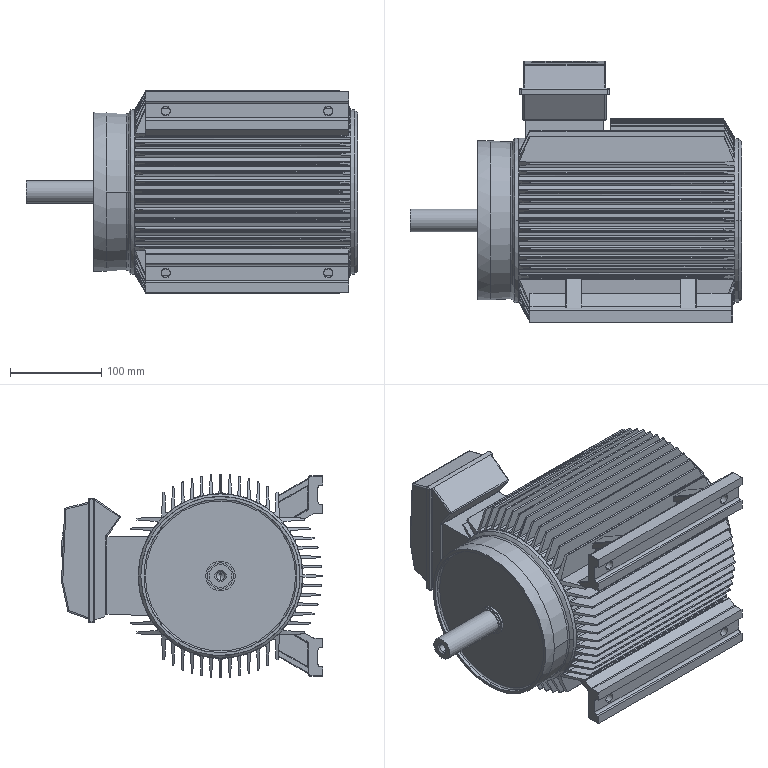Part | NX | 1 solid | 679 faces | box 362.6 x 286.311 x 222.656 mm | volume 9083638 mm3 | cylinder 330 | plane 270 | cone 22 | torus 22 | spline 21 | sphere 14 | commonest cylinder face diameters 3.136 x110 1.4 x45 180.006 x44 2.8 x31 0.627 x14 1.593 x10